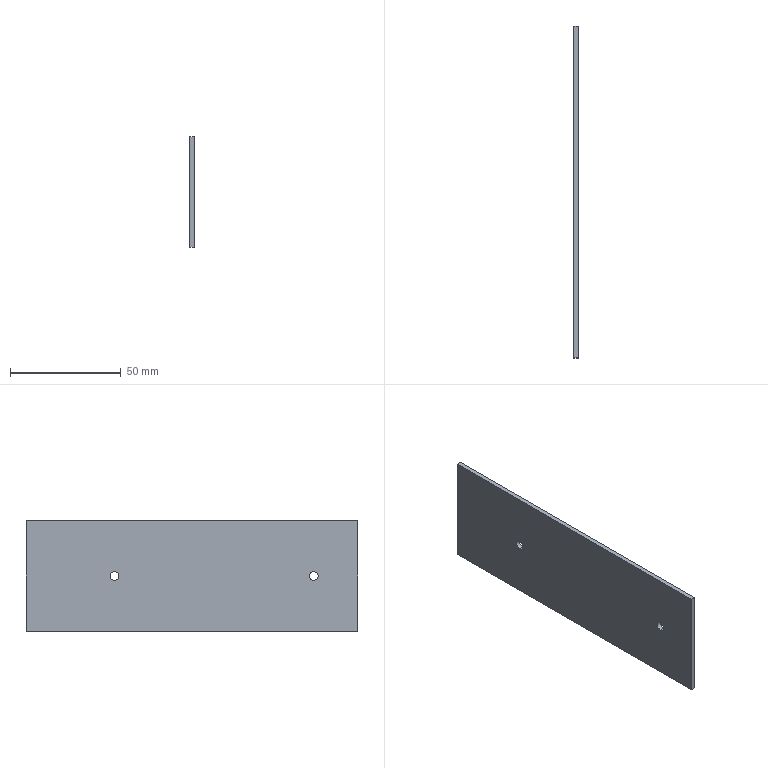Part | SolidWorks | features ICE 3, Extrusion 1 | 1 solid | 10 faces | box 2 x 150 x 50 mm | volume 14950 mm3 | plane 6 | cylinder 4 | commonest cylinder face diameters 4 x4
STEP:
#1=CARTESIAN_POINT('',(-1.,50.,27.));
#2=VERTEX_POINT('',#1);
#3=CARTESIAN_POINT('',(-1.,50.,23.));
#4=VERTEX_POINT('',#3);
#5=CARTESIAN_POINT('',(-1.,50.,25.));
#6=DIRECTION('',(1.,0.,0.));
#7=DIRECTION('',(0.,0.,-1.));
#8=AXIS2_PLACEMENT_3D('',#5,#6,#7);
#9=CIRCLE('',#8,2.);
#10=EDGE_CURVE('',#2,#4,#9,.T.);
#11=ORIENTED_EDGE('',*,*,#10,.F.);
#12=CARTESIAN_POINT('',(1.,50.,27.));
#13=VERTEX_POINT('',#12);
#14=CARTESIAN_POINT('',(-9.,50.,27.));
#15=DIRECTION('',(1.,0.,0.));
#16=VECTOR('',#15,1000.);
#17=LINE('',#14,#16);
#18=EDGE_CURVE('',#2,#13,#17,.T.);
#19=ORIENTED_EDGE('',*,*,#18,.T.);
#20=CARTESIAN_POINT('',(1.,50.,23.));
#21=VERTEX_POINT('',#20);
#22=CARTESIAN_POINT('',(1.,50.,25.));
#23=DIRECTION('',(1.,0.,0.));
#24=DIRECTION('',(0.,0.,-1.));
#25=AXIS2_PLACEMENT_3D('',#22,#23,#24);
#26=CIRCLE('',#25,2.);
#27=EDGE_CURVE('',#13,#21,#26,.T.);
#28=ORIENTED_EDGE('',*,*,#27,.T.);
#29=CARTESIAN_POINT('',(-9.,50.,23.));
#30=DIRECTION('',(1.,0.,0.));
#31=VECTOR('',#30,1000.);
#32=LINE('',#29,#31);
#33=EDGE_CURVE('',#4,#21,#32,.T.);
#34=ORIENTED_EDGE('',*,*,#33,.F.);
#35=EDGE_LOOP('',(#11,#19,#28,#34));
#36=FACE_OUTER_BOUND('',#35,.T.);
#37=CARTESIAN_POINT('',(-9.,50.,25.));
#38=DIRECTION('',(1.,0.,0.));
#39=DIRECTION('',(0.,0.,-1.));
#40=AXIS2_PLACEMENT_3D('',#37,#38,#39);
#41=CYLINDRICAL_SURFACE('',#40,2.);
#42=ADVANCED_FACE('',(#36),#41,.F.);
#43=CARTESIAN_POINT('',(-1.,-40.,27.));
#44=VERTEX_POINT('',#43);
#45=CARTESIAN_POINT('',(-1.,-40.,23.));
#46=VERTEX_POINT('',#45);
#47=CARTESIAN_POINT('',(-1.,-40.,25.));
#48=DIRECTION('',(1.,0.,0.));
#49=DIRECTION('',(0.,0.,-1.));
#50=AXIS2_PLACEMENT_3D('',#47,#48,#49);
#51=CIRCLE('',#50,2.);
#52=EDGE_CURVE('',#44,#46,#51,.T.);
#53=ORIENTED_EDGE('',*,*,#52,.F.);
#54=CARTESIAN_POINT('',(1.,-40.,27.));
#55=VERTEX_POINT('',#54);
#56=CARTESIAN_POINT('',(-19.,-40.,27.));
#57=DIRECTION('',(1.,0.,0.));
#58=VECTOR('',#57,1000.);
#59=LINE('',#56,#58);
#60=EDGE_CURVE('',#44,#55,#59,.T.);
#61=ORIENTED_EDGE('',*,*,#60,.T.);
#62=CARTESIAN_POINT('',(1.,-40.,23.));
#63=VERTEX_POINT('',#62);
#64=CARTESIAN_POINT('',(1.,-40.,25.));
#65=DIRECTION('',(1.,0.,0.));
#66=DIRECTION('',(0.,0.,-1.));
#67=AXIS2_PLACEMENT_3D('',#64,#65,#66);
#68=CIRCLE('',#67,2.);
#69=EDGE_CURVE('',#55,#63,#68,.T.);
#70=ORIENTED_EDGE('',*,*,#69,.T.);
#71=CARTESIAN_POINT('',(-19.,-40.,23.));
#72=DIRECTION('',(1.,0.,0.));
#73=VECTOR('',#72,1000.);
#74=LINE('',#71,#73);
#75=EDGE_CURVE('',#46,#63,#74,.T.);
#76=ORIENTED_EDGE('',*,*,#75,.F.);
#77=EDGE_LOOP('',(#53,#61,#70,#76));
#78=FACE_OUTER_BOUND('',#77,.T.);
#79=CARTESIAN_POINT('',(-19.,-40.,25.));
#80=DIRECTION('',(1.,0.,0.));
#81=DIRECTION('',(0.,0.,-1.));
#82=AXIS2_PLACEMENT_3D('',#79,#80,#81);
#83=CYLINDRICAL_SURFACE('',#82,2.);
#84=ADVANCED_FACE('',(#78),#83,.F.);
#85=CARTESIAN_POINT('',(1.,50.,25.));
#86=DIRECTION('',(1.,0.,0.));
#87=DIRECTION('',(0.,0.,-1.));
#88=AXIS2_PLACEMENT_3D('',#85,#86,#87);
#89=CIRCLE('',#88,2.);
#90=EDGE_CURVE('',#21,#13,#89,.T.);
#91=ORIENTED_EDGE('',*,*,#90,.F.);
#92=ORIENTED_EDGE('',*,*,#27,.F.);
#93=EDGE_LOOP('',(#91,#92));
#94=FACE_BOUND('',#93,.T.);
#95=CARTESIAN_POINT('',(1.,-40.,25.));
#96=DIRECTION('',(1.,0.,0.));
#97=DIRECTION('',(0.,0.,-1.));
#98=AXIS2_PLACEMENT_3D('',#95,#96,#97);
#99=CIRCLE('',#98,2.);
#100=EDGE_CURVE('',#63,#55,#99,.T.);
#101=ORIENTED_EDGE('',*,*,#100,.F.);
#102=ORIENTED_EDGE('',*,*,#69,.F.);
#103=EDGE_LOOP('',(#101,#102));
#104=FACE_BOUND('',#103,.T.);
#105=CARTESIAN_POINT('',(1.,-60.,50.));
#106=VERTEX_POINT('',#105);
#107=CARTESIAN_POINT('',(1.,90.,50.));
#108=VERTEX_POINT('',#107);
#109=CARTESIAN_POINT('',(1.,-90.,50.));
#110=DIRECTION('',(0.,1.,0.));
#111=VECTOR('',#110,1000.);
#112=LINE('',#109,#111);
#113=EDGE_CURVE('',#106,#108,#112,.T.);
#114=ORIENTED_EDGE('',*,*,#113,.F.);
#115=CARTESIAN_POINT('',(1.,-60.,0.));
#116=VERTEX_POINT('',#115);
#117=CARTESIAN_POINT('',(1.,-60.,50.));
#118=DIRECTION('',(0.,0.,-1.));
#119=VECTOR('',#118,1000.);
#120=LINE('',#117,#119);
#121=EDGE_CURVE('',#106,#116,#120,.T.);
#122=ORIENTED_EDGE('',*,*,#121,.T.);
#123=CARTESIAN_POINT('',(1.,90.,0.));
#124=VERTEX_POINT('',#123);
#125=CARTESIAN_POINT('',(1.,-90.,0.));
#126=DIRECTION('',(0.,1.,0.));
#127=VECTOR('',#126,1000.);
#128=LINE('',#125,#127);
#129=EDGE_CURVE('',#116,#124,#128,.T.);
#130=ORIENTED_EDGE('',*,*,#129,.T.);
#131=CARTESIAN_POINT('',(1.,90.,50.));
#132=DIRECTION('',(0.,0.,-1.));
#133=VECTOR('',#132,1000.);
#134=LINE('',#131,#133);
#135=EDGE_CURVE('',#108,#124,#134,.T.);
#136=ORIENTED_EDGE('',*,*,#135,.F.);
#137=EDGE_LOOP('',(#114,#122,#130,#136));
#138=FACE_OUTER_BOUND('',#137,.T.);
#139=CARTESIAN_POINT('',(1.,-90.,50.));
#140=DIRECTION('',(-1.,0.,0.));
#141=DIRECTION('',(0.,0.,1.));
#142=AXIS2_PLACEMENT_3D('',#139,#140,#141);
#143=PLANE('',#142);
#144=ADVANCED_FACE('',(#94,#104,#138),#143,.F.);
#145=CARTESIAN_POINT('',(-1.,90.,0.));
#146=VERTEX_POINT('',#145);
#147=CARTESIAN_POINT('',(-1.,90.,0.));
#148=DIRECTION('',(-1.,0.,0.));
#149=VECTOR('',#148,1000.);
#150=LINE('',#147,#149);
#151=EDGE_CURVE('',#124,#146,#150,.T.);
#152=ORIENTED_EDGE('',*,*,#151,.T.);
#153=CARTESIAN_POINT('',(-1.,90.,50.));
#154=VERTEX_POINT('',#153);
#155=CARTESIAN_POINT('',(-1.,90.,50.));
#156=DIRECTION('',(0.,0.,-1.));
#157=VECTOR('',#156,1000.);
#158=LINE('',#155,#157);
#159=EDGE_CURVE('',#154,#146,#158,.T.);
#160=ORIENTED_EDGE('',*,*,#159,.F.);
#161=CARTESIAN_POINT('',(-1.,90.,50.));
#162=DIRECTION('',(-1.,0.,0.));
#163=VECTOR('',#162,1000.);
#164=LINE('',#161,#163);
#165=EDGE_CURVE('',#108,#154,#164,.T.);
#166=ORIENTED_EDGE('',*,*,#165,.F.);
#167=ORIENTED_EDGE('',*,*,#135,.T.);
#168=EDGE_LOOP('',(#152,#160,#166,#167));
#169=FACE_OUTER_BOUND('',#168,.T.);
#170=CARTESIAN_POINT('',(-1.,90.,50.));
#171=DIRECTION('',(0.,-1.,0.));
#172=DIRECTION('',(0.,0.,-1.));
#173=AXIS2_PLACEMENT_3D('',#170,#171,#172);
#174=PLANE('',#173);
#175=ADVANCED_FACE('',(#169),#174,.F.);
#176=CARTESIAN_POINT('',(-1.,50.,25.));
#177=DIRECTION('',(1.,0.,0.));
#178=DIRECTION('',(0.,0.,-1.));
#179=AXIS2_PLACEMENT_3D('',#176,#177,#178);
#180=CIRCLE('',#179,2.);
#181=EDGE_CURVE('',#4,#2,#180,.T.);
#182=ORIENTED_EDGE('',*,*,#181,.T.);
#183=ORIENTED_EDGE('',*,*,#10,.T.);
#184=EDGE_LOOP('',(#182,#183));
#185=FACE_BOUND('',#184,.T.);
#186=CARTESIAN_POINT('',(-1.,-40.,25.));
#187=DIRECTION('',(1.,0.,0.));
#188=DIRECTION('',(0.,0.,-1.));
#189=AXIS2_PLACEMENT_3D('',#186,#187,#188);
#190=CIRCLE('',#189,2.);
#191=EDGE_CURVE('',#46,#44,#190,.T.);
#192=ORIENTED_EDGE('',*,*,#191,.T.);
#193=ORIENTED_EDGE('',*,*,#52,.T.);
#194=EDGE_LOOP('',(#192,#193));
#195=FACE_BOUND('',#194,.T.);
#196=CARTESIAN_POINT('',(-1.,-60.,0.));
#197=VERTEX_POINT('',#196);
#198=CARTESIAN_POINT('',(-1.,-90.,0.));
#199=DIRECTION('',(0.,-1.,0.));
#200=VECTOR('',#199,1000.);
#201=LINE('',#198,#200);
#202=EDGE_CURVE('',#146,#197,#201,.T.);
#203=ORIENTED_EDGE('',*,*,#202,.T.);
#204=CARTESIAN_POINT('',(-1.,-60.,50.));
#205=VERTEX_POINT('',#204);
#206=CARTESIAN_POINT('',(-1.,-60.,151.533));
#207=DIRECTION('',(0.,0.,-1.));
#208=VECTOR('',#207,1000.);
#209=LINE('',#206,#208);
#210=EDGE_CURVE('',#205,#197,#209,.T.);
#211=ORIENTED_EDGE('',*,*,#210,.F.);
#212=CARTESIAN_POINT('',(-1.,-90.,50.));
#213=DIRECTION('',(0.,-1.,0.));
#214=VECTOR('',#213,1000.);
#215=LINE('',#212,#214);
#216=EDGE_CURVE('',#154,#205,#215,.T.);
#217=ORIENTED_EDGE('',*,*,#216,.F.);
#218=ORIENTED_EDGE('',*,*,#159,.T.);
#219=EDGE_LOOP('',(#203,#211,#217,#218));
#220=FACE_OUTER_BOUND('',#219,.T.);
#221=CARTESIAN_POINT('',(-1.,-90.,50.));
#222=DIRECTION('',(1.,0.,0.));
#223=DIRECTION('',(0.,0.,-1.));
#224=AXIS2_PLACEMENT_3D('',#221,#222,#223);
#225=PLANE('',#224);
#226=ADVANCED_FACE('',(#185,#195,#220),#225,.F.);
#227=ORIENTED_EDGE('',*,*,#216,.T.);
#228=CARTESIAN_POINT('',(0.,-60.,50.));
#229=DIRECTION('',(1.,0.,0.));
#230=VECTOR('',#229,1000.);
#231=LINE('',#228,#230);
#232=EDGE_CURVE('',#205,#106,#231,.T.);
#233=ORIENTED_EDGE('',*,*,#232,.T.);
#234=ORIENTED_EDGE('',*,*,#113,.T.);
#235=ORIENTED_EDGE('',*,*,#165,.T.);
#236=EDGE_LOOP('',(#227,#233,#234,#235));
#237=FACE_OUTER_BOUND('',#236,.T.);
#238=CARTESIAN_POINT('',(0.,0.,50.));
#239=DIRECTION('',(0.,0.,-1.));
#240=DIRECTION('',(-1.,0.,0.));
#241=AXIS2_PLACEMENT_3D('',#238,#239,#240);
#242=PLANE('',#241);
#243=ADVANCED_FACE('',(#237),#242,.F.);
#244=CARTESIAN_POINT('',(0.,-60.,0.));
#245=DIRECTION('',(1.,0.,0.));
#246=VECTOR('',#245,1000.);
#247=LINE('',#244,#246);
#248=EDGE_CURVE('',#197,#116,#247,.T.);
#249=ORIENTED_EDGE('',*,*,#248,.F.);
#250=ORIENTED_EDGE('',*,*,#202,.F.);
#251=ORIENTED_EDGE('',*,*,#151,.F.);
#252=ORIENTED_EDGE('',*,*,#129,.F.);
#253=EDGE_LOOP('',(#249,#250,#251,#252));
#254=FACE_OUTER_BOUND('',#253,.T.);
#255=CARTESIAN_POINT('',(0.,0.,0.));
#256=DIRECTION('',(0.,0.,-1.));
#257=DIRECTION('',(-1.,0.,0.));
#258=AXIS2_PLACEMENT_3D('',#255,#256,#257);
#259=PLANE('',#258);
#260=ADVANCED_FACE('',(#254),#259,.T.);
#261=ORIENTED_EDGE('',*,*,#60,.F.);
#262=ORIENTED_EDGE('',*,*,#191,.F.);
#263=ORIENTED_EDGE('',*,*,#75,.T.);
#264=ORIENTED_EDGE('',*,*,#100,.T.);
#265=EDGE_LOOP('',(#261,#262,#263,#264));
#266=FACE_OUTER_BOUND('',#265,.T.);
#267=CARTESIAN_POINT('',(-19.,-40.,25.));
#268=DIRECTION('',(1.,0.,0.));
#269=DIRECTION('',(0.,0.,-1.));
#270=AXIS2_PLACEMENT_3D('',#267,#268,#269);
#271=CYLINDRICAL_SURFACE('',#270,2.);
#272=ADVANCED_FACE('',(#266),#271,.F.);
#273=ORIENTED_EDGE('',*,*,#18,.F.);
#274=ORIENTED_EDGE('',*,*,#181,.F.);
#275=ORIENTED_EDGE('',*,*,#33,.T.);
#276=ORIENTED_EDGE('',*,*,#90,.T.);
#277=EDGE_LOOP('',(#273,#274,#275,#276));
#278=FACE_OUTER_BOUND('',#277,.T.);
#279=CARTESIAN_POINT('',(-9.,50.,25.));
#280=DIRECTION('',(1.,0.,0.));
#281=DIRECTION('',(0.,0.,-1.));
#282=AXIS2_PLACEMENT_3D('',#279,#280,#281);
#283=CYLINDRICAL_SURFACE('',#282,2.);
#284=ADVANCED_FACE('',(#278),#283,.F.);
#285=ORIENTED_EDGE('',*,*,#210,.T.);
#286=ORIENTED_EDGE('',*,*,#248,.T.);
#287=ORIENTED_EDGE('',*,*,#121,.F.);
#288=ORIENTED_EDGE('',*,*,#232,.F.);
#289=EDGE_LOOP('',(#285,#286,#287,#288));
#290=FACE_OUTER_BOUND('',#289,.T.);
#291=CARTESIAN_POINT('',(9.,-60.,151.533));
#292=DIRECTION('',(0.,1.,0.));
#293=DIRECTION('',(0.,0.,1.));
#294=AXIS2_PLACEMENT_3D('',#291,#292,#293);
#295=PLANE('',#294);
#296=ADVANCED_FACE('',(#290),#295,.F.);
#297=CLOSED_SHELL('',(#42,#84,#144,#175,#226,#243,#260,#272,#284,#296));
#298=MANIFOLD_SOLID_BREP('',#297);
#299=CARTESIAN_POINT('',(0.,0.,0.));
#300=DIRECTION('',(0.,0.,1.));
#301=DIRECTION('',(1.,0.,0.));
#302=AXIS2_PLACEMENT_3D('',#299,#300,#301);
#303=(LENGTH_UNIT()NAMED_UNIT(*)SI_UNIT(.MILLI.,.METRE.));
#304=UNCERTAINTY_MEASURE_WITH_UNIT(LENGTH_MEASURE(0.00001),#303,'','');
#305=(NAMED_UNIT(*)PLANE_ANGLE_UNIT()SI_UNIT($,.RADIAN.));
#306=(NAMED_UNIT(*)SI_UNIT($,.STERADIAN.)SOLID_ANGLE_UNIT());
#307=(GEOMETRIC_REPRESENTATION_CONTEXT(3)GLOBAL_UNCERTAINTY_ASSIGNED_CONTEXT((#304))GLOBAL_UNIT_ASSIGNED_CONTEXT((#303,#305,#306))REPRESENTATION_CONTEXT('',''));
#308=ADVANCED_BREP_SHAPE_REPRESENTATION('',(#298,#302),#307);